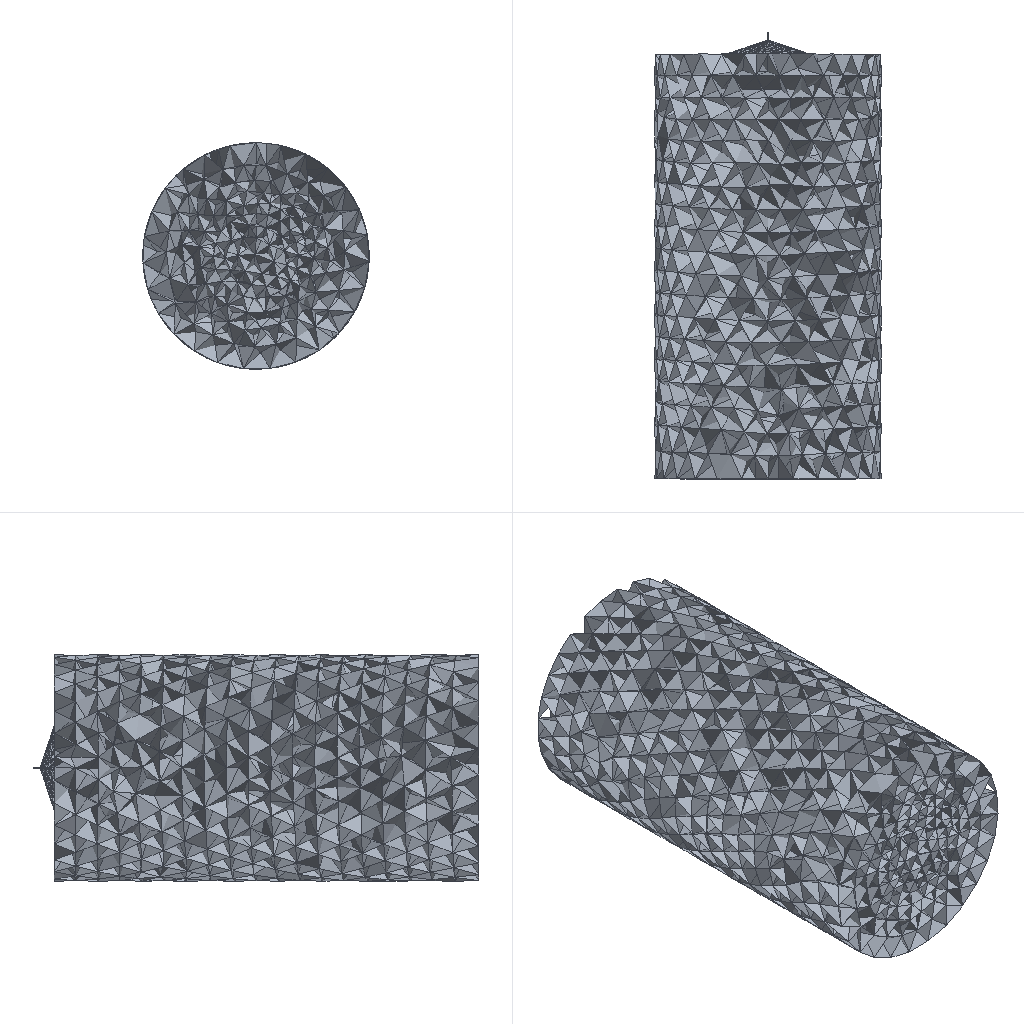Simulation study | ansys fluent
Set-up summary:
category,name,step,type,value,unit,region
solver,ansys_fluent,,Fluent 26.1.0
units,SI m-kg-s (Fluent internal),,stated,boundary values in the units shown in brackets; results in listed units
analysis,deck.cas,,cfd steady,"dimension=3D; solver=3d, dp, pbns, vof, sstkw (3d, double precision, pressure-based, VOF, SST k-omega); source_case=.cas"
model,Space,deck.cas,,3D
model,Time,deck.cas,,Steady
model,Viscous,deck.cas,,SST k-omega turbulence model
model,Heat Transfer,deck.cas,,Disabled
model,Multiphase,deck.cas,,Volume of Fluid
mesh,nodes,,,23238
mesh,elements,,,106734
mesh,faces,,,223141
cell_zone,__-__ (mixture),deck.cas,fluid,material=water-liquid,,zone 3
cell_zone,__-__ (air),deck.cas,fluid,material=air,,zone 3
cell_zone,__-__ (water),deck.cas,fluid,material=water-liquid,,zone 3
material,water-liquid (fluid),,Density,998.2,kg/m^3
material,water-liquid (fluid),,Viscosity,0.001003,kg/(m s)
material,air (fluid),,Density,1.225,kg/m^3
material,air (fluid),,Viscosity,1.7894e-05,kg/(m s)
material,aluminum (solid),,Density,2719,kg/m^3
bc,int (mixture),deck.cas,pressure-inlet,Gauge Total Pressure [Pa]=50000000; Supersonic/Initial Gauge Pressure [Pa]=50000000,,zone 5
bc,int (air),deck.cas,pressure-inlet,,,zone 5
bc,int (water),deck.cas,pressure-inlet,Volume Fraction=1,,zone 5
bc,wall (mixture),deck.cas,wall,Wall Motion=Stationary Wall; Shear Boundary Condition=No Slip; Wall Surface Roughness=Standard,,zone 6
bc,wall (air),deck.cas,wall,,,zone 6
bc,wall (water),deck.cas,wall,,,zone 6
bc,out (mixture),deck.cas,pressure-outlet,Backflow Direction Specification Method=Normal to Boundary,,zone 7
bc,out (air),deck.cas,pressure-outlet,,,zone 7
bc,out (water),deck.cas,pressure-outlet,,,zone 7
Results summary:
result,mass flow rate int,deck.cas,,0.000128,kg/s
result,mass flow rate out,deck.cas,,-1.45698e-06,kg/s
result,mass flow rate wall,deck.cas,,-0,kg/s
result,mass flow rate Net,deck.cas,,0.0001266,kg/s
result,wall force total wall,deck.cas,,"(-3.4888e-05, -0.06275, -1.49222e-05)",N
result,wall force pressure wall,deck.cas,,"(-6.71144e-05, -0.02514, -5.26522e-05)",N
result,wall force viscous wall,deck.cas,,"(3.22264e-05, -0.03761, 3.773e-05)",N
result,wall force total Net,deck.cas,,"(-3.4888e-05, -0.06275, -1.49222e-05)",N
result,wall force pressure Net,deck.cas,,"(-6.71144e-05, -0.02514, -5.26522e-05)",N
result,wall force viscous Net,deck.cas,,"(3.22264e-05, -0.03761, 3.773e-05)",N